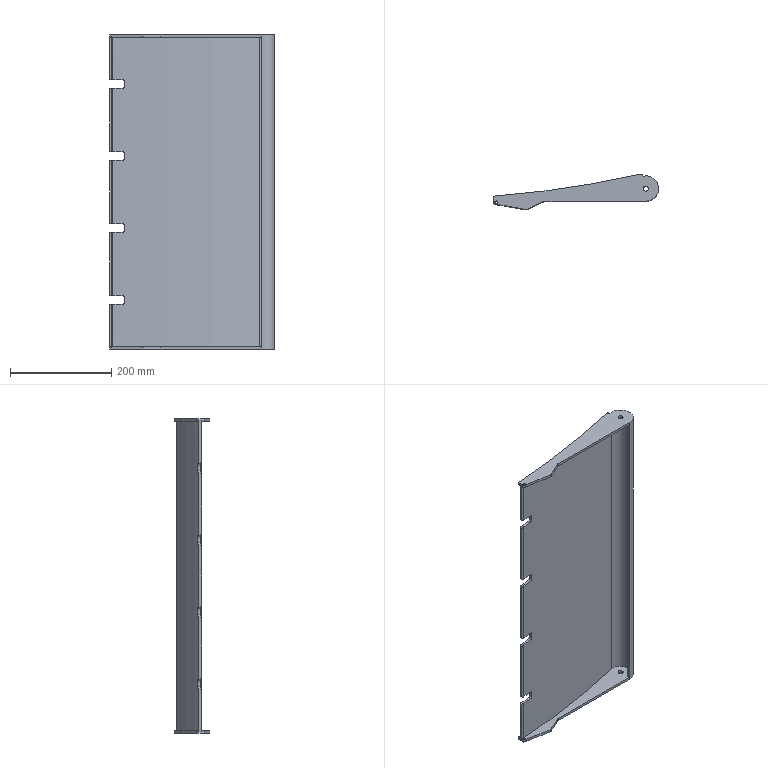Part | SolidWorks | features Fillet 3, ICE 3, Extrusion 1, MirrorPattern 1, Shell 1 | 1 solid | 83 faces | box 325.159 x 69.885 x 620 mm | volume 1237275 mm3 | cylinder 49 | plane 34 | commonest cylinder face diameters 6 x21 10 x10 5 x7 4010 x6 3990 x2 40 x1